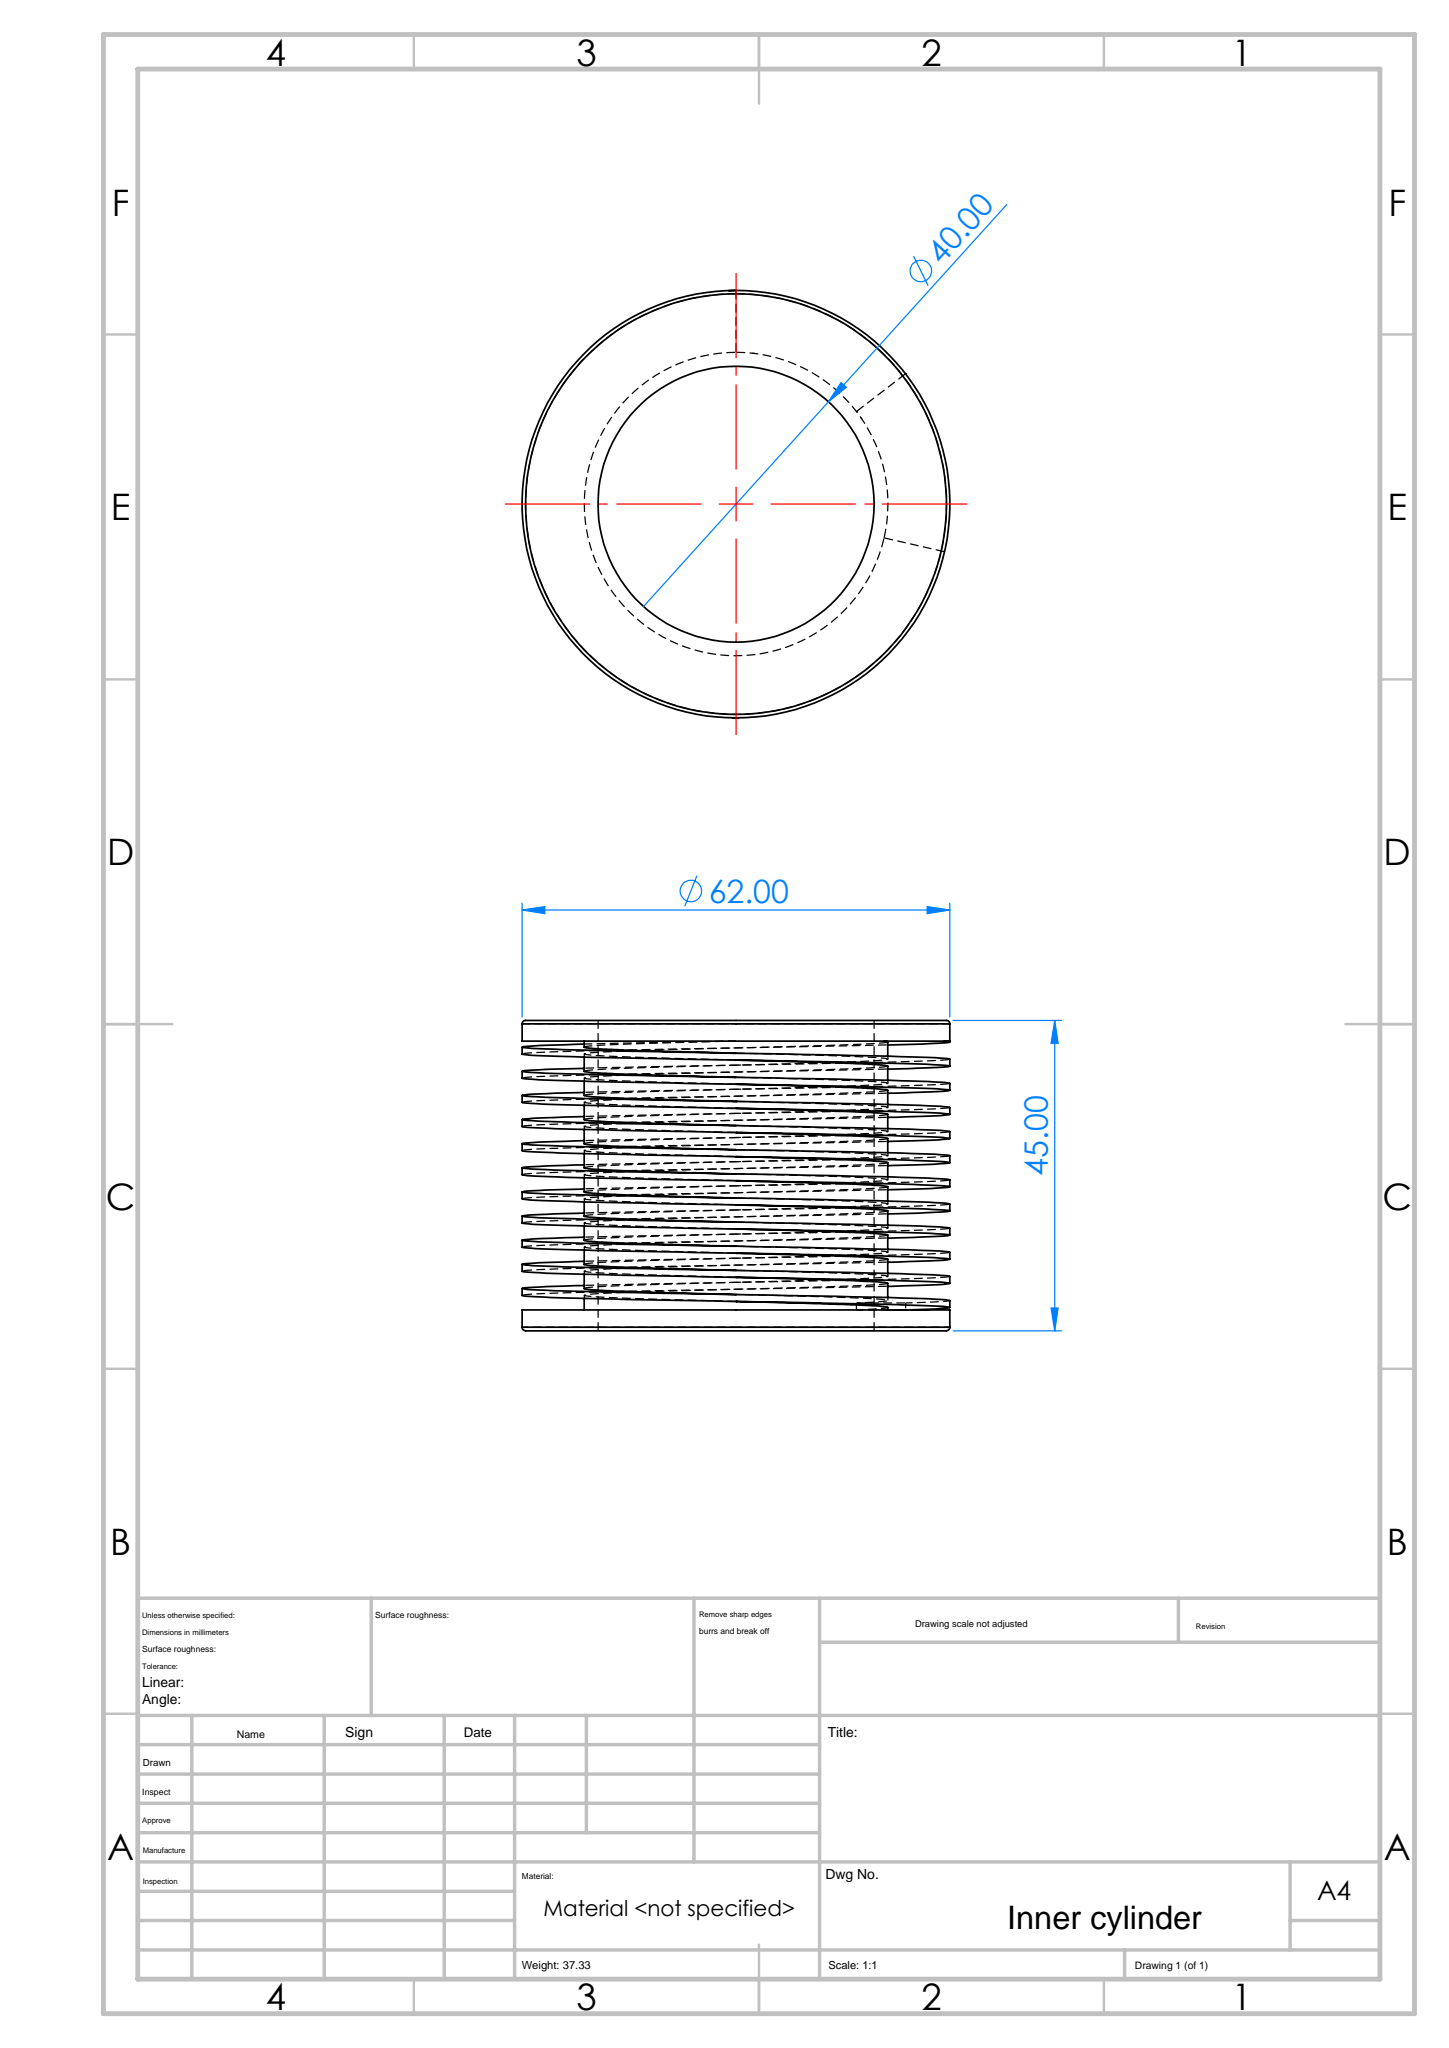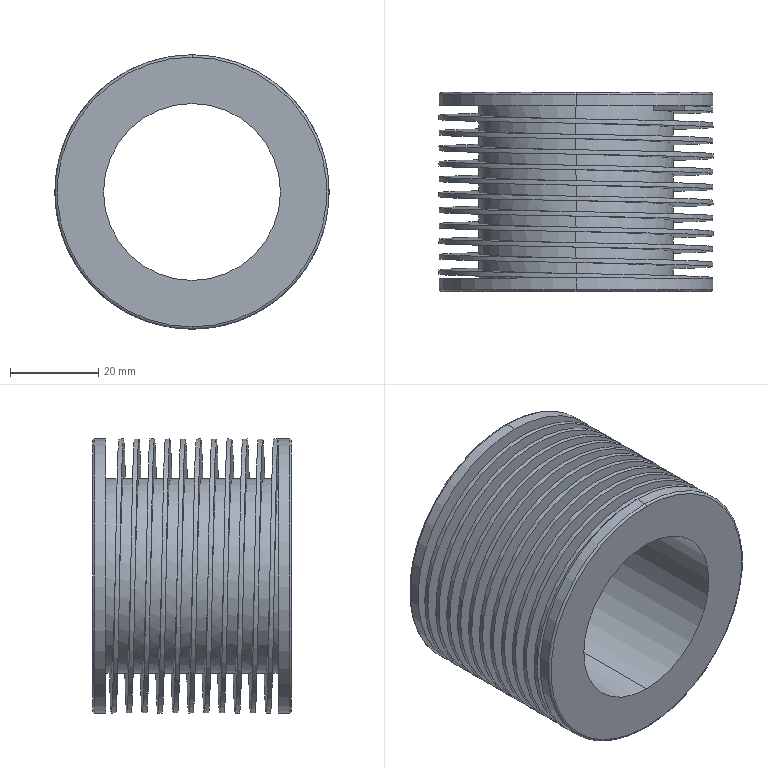Part | SolidWorks | features Fillet 2, Helix 1, Revolution 1, Sweep 1 | 1 solid | 42 faces | box 62 x 45 x 62 mm | volume 37551 mm3 | cylinder 30 | plane 5 | torus 4 | spline 3 | commonest cylinder face diameters 44 x24 62 x4 40 x2